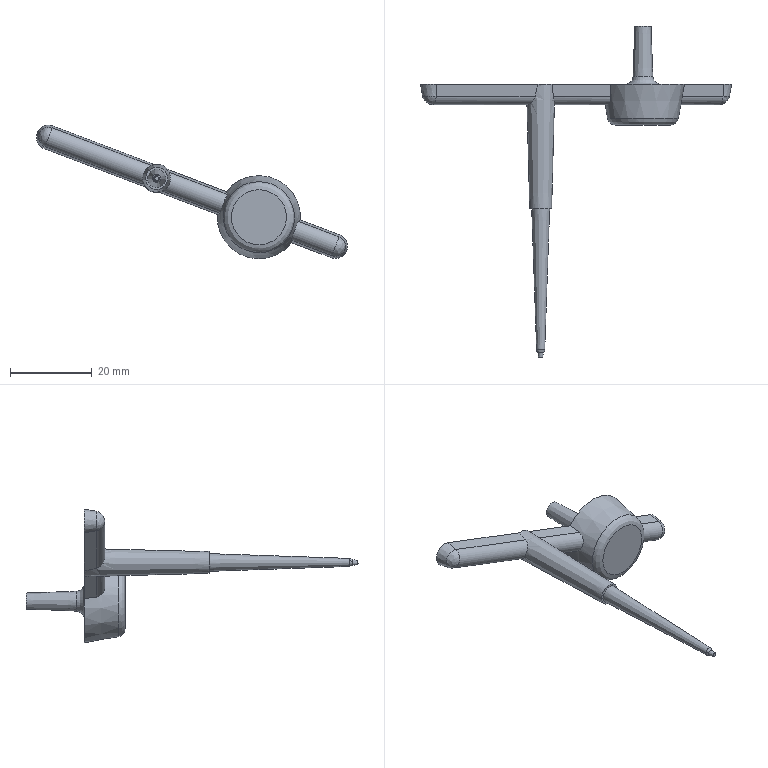Part | STEP file | RUNNER_id158_x_t | 1 solid | 31 faces | box 76.069 x 81.16 x 32.686 mm | volume 5385 mm3 | plane 10 | cone 8 | other 7 | cylinder 4 | spline 2 | commonest cylinder face diameters 5 x3 47.337 x1